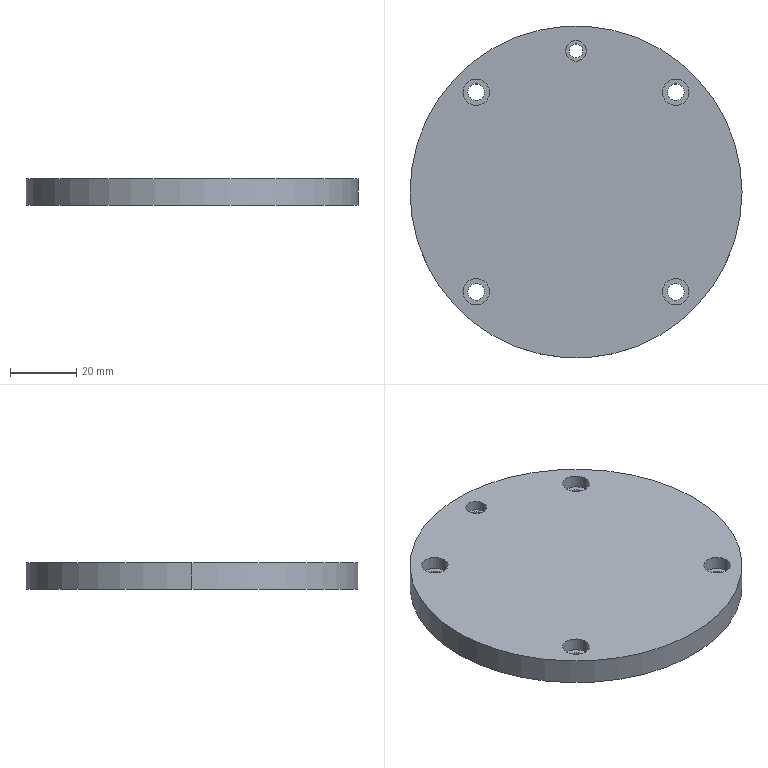Part | SolidWorks | features ICE 4, Extrusion 1 | 1 solid | 29 faces | box 100 x 100 x 8 mm | volume 61554 mm3 | cylinder 22 | plane 7 | commonest cylinder face diameters 5 x8 8 x8 4.2 x2 6.2 x2 100 x2
STEP:
#1=CARTESIAN_POINT('',(-2.1,42.5,0.));
#2=VERTEX_POINT('',#1);
#3=CARTESIAN_POINT('',(2.1,42.5,0.));
#4=VERTEX_POINT('',#3);
#5=CARTESIAN_POINT('',(0.,42.5,0.));
#6=DIRECTION('',(0.,0.,1.));
#7=DIRECTION('',(1.,0.,0.));
#8=AXIS2_PLACEMENT_3D('',#5,#6,#7);
#9=CIRCLE('',#8,2.1);
#10=EDGE_CURVE('',#2,#4,#9,.T.);
#11=ORIENTED_EDGE('',*,*,#10,.F.);
#12=CARTESIAN_POINT('',(-2.1,42.5,5.));
#13=VERTEX_POINT('',#12);
#14=CARTESIAN_POINT('',(-2.1,42.5,0.));
#15=DIRECTION('',(0.,0.,1.));
#16=VECTOR('',#15,1000.);
#17=LINE('',#14,#16);
#18=EDGE_CURVE('',#2,#13,#17,.T.);
#19=ORIENTED_EDGE('',*,*,#18,.T.);
#20=CARTESIAN_POINT('',(2.1,42.5,5.));
#21=VERTEX_POINT('',#20);
#22=CARTESIAN_POINT('',(0.,42.5,5.));
#23=DIRECTION('',(0.,0.,1.));
#24=DIRECTION('',(1.,0.,0.));
#25=AXIS2_PLACEMENT_3D('',#22,#23,#24);
#26=CIRCLE('',#25,2.1);
#27=EDGE_CURVE('',#13,#21,#26,.T.);
#28=ORIENTED_EDGE('',*,*,#27,.T.);
#29=CARTESIAN_POINT('',(2.1,42.5,0.));
#30=DIRECTION('',(0.,0.,1.));
#31=VECTOR('',#30,1000.);
#32=LINE('',#29,#31);
#33=EDGE_CURVE('',#4,#21,#32,.T.);
#34=ORIENTED_EDGE('',*,*,#33,.F.);
#35=EDGE_LOOP('',(#11,#19,#28,#34));
#36=FACE_OUTER_BOUND('',#35,.T.);
#37=CARTESIAN_POINT('',(0.,42.5,0.));
#38=DIRECTION('',(0.,0.,1.));
#39=DIRECTION('',(1.,0.,0.));
#40=AXIS2_PLACEMENT_3D('',#37,#38,#39);
#41=CYLINDRICAL_SURFACE('',#40,2.1);
#42=ADVANCED_FACE('',(#36),#41,.F.);
#43=CARTESIAN_POINT('',(27.554,-30.05,0.));
#44=VERTEX_POINT('',#43);
#45=CARTESIAN_POINT('',(32.554,-30.05,0.));
#46=VERTEX_POINT('',#45);
#47=CARTESIAN_POINT('',(30.054,-30.05,0.));
#48=DIRECTION('',(0.,0.,1.));
#49=DIRECTION('',(1.,0.,0.));
#50=AXIS2_PLACEMENT_3D('',#47,#48,#49);
#51=CIRCLE('',#50,2.5);
#52=EDGE_CURVE('',#44,#46,#51,.T.);
#53=ORIENTED_EDGE('',*,*,#52,.F.);
#54=CARTESIAN_POINT('',(27.554,-30.05,4.));
#55=VERTEX_POINT('',#54);
#56=CARTESIAN_POINT('',(27.554,-30.05,0.));
#57=DIRECTION('',(0.,0.,1.));
#58=VECTOR('',#57,1000.);
#59=LINE('',#56,#58);
#60=EDGE_CURVE('',#44,#55,#59,.T.);
#61=ORIENTED_EDGE('',*,*,#60,.T.);
#62=CARTESIAN_POINT('',(32.554,-30.05,4.));
#63=VERTEX_POINT('',#62);
#64=CARTESIAN_POINT('',(30.054,-30.05,4.));
#65=DIRECTION('',(0.,0.,1.));
#66=DIRECTION('',(1.,0.,0.));
#67=AXIS2_PLACEMENT_3D('',#64,#65,#66);
#68=CIRCLE('',#67,2.5);
#69=EDGE_CURVE('',#55,#63,#68,.T.);
#70=ORIENTED_EDGE('',*,*,#69,.T.);
#71=CARTESIAN_POINT('',(32.554,-30.05,0.));
#72=DIRECTION('',(0.,0.,1.));
#73=VECTOR('',#72,1000.);
#74=LINE('',#71,#73);
#75=EDGE_CURVE('',#46,#63,#74,.T.);
#76=ORIENTED_EDGE('',*,*,#75,.F.);
#77=EDGE_LOOP('',(#53,#61,#70,#76));
#78=FACE_OUTER_BOUND('',#77,.T.);
#79=CARTESIAN_POINT('',(30.054,-30.05,0.));
#80=DIRECTION('',(0.,0.,1.));
#81=DIRECTION('',(1.,0.,0.));
#82=AXIS2_PLACEMENT_3D('',#79,#80,#81);
#83=CYLINDRICAL_SURFACE('',#82,2.5);
#84=ADVANCED_FACE('',(#78),#83,.F.);
#85=CARTESIAN_POINT('',(-32.554,-30.05,0.));
#86=VERTEX_POINT('',#85);
#87=CARTESIAN_POINT('',(-27.554,-30.05,0.));
#88=VERTEX_POINT('',#87);
#89=CARTESIAN_POINT('',(-30.054,-30.05,0.));
#90=DIRECTION('',(0.,0.,1.));
#91=DIRECTION('',(1.,0.,0.));
#92=AXIS2_PLACEMENT_3D('',#89,#90,#91);
#93=CIRCLE('',#92,2.5);
#94=EDGE_CURVE('',#86,#88,#93,.T.);
#95=ORIENTED_EDGE('',*,*,#94,.F.);
#96=CARTESIAN_POINT('',(-32.554,-30.05,4.));
#97=VERTEX_POINT('',#96);
#98=CARTESIAN_POINT('',(-32.554,-30.05,0.));
#99=DIRECTION('',(0.,0.,1.));
#100=VECTOR('',#99,1000.);
#101=LINE('',#98,#100);
#102=EDGE_CURVE('',#86,#97,#101,.T.);
#103=ORIENTED_EDGE('',*,*,#102,.T.);
#104=CARTESIAN_POINT('',(-27.554,-30.05,4.));
#105=VERTEX_POINT('',#104);
#106=CARTESIAN_POINT('',(-30.054,-30.05,4.));
#107=DIRECTION('',(0.,0.,1.));
#108=DIRECTION('',(1.,0.,0.));
#109=AXIS2_PLACEMENT_3D('',#106,#107,#108);
#110=CIRCLE('',#109,2.5);
#111=EDGE_CURVE('',#97,#105,#110,.T.);
#112=ORIENTED_EDGE('',*,*,#111,.T.);
#113=CARTESIAN_POINT('',(-27.554,-30.05,0.));
#114=DIRECTION('',(0.,0.,1.));
#115=VECTOR('',#114,1000.);
#116=LINE('',#113,#115);
#117=EDGE_CURVE('',#88,#105,#116,.T.);
#118=ORIENTED_EDGE('',*,*,#117,.F.);
#119=EDGE_LOOP('',(#95,#103,#112,#118));
#120=FACE_OUTER_BOUND('',#119,.T.);
#121=CARTESIAN_POINT('',(-30.054,-30.05,0.));
#122=DIRECTION('',(0.,0.,1.));
#123=DIRECTION('',(1.,0.,0.));
#124=AXIS2_PLACEMENT_3D('',#121,#122,#123);
#125=CYLINDRICAL_SURFACE('',#124,2.5);
#126=ADVANCED_FACE('',(#120),#125,.F.);
#127=CARTESIAN_POINT('',(27.554,30.05,0.));
#128=VERTEX_POINT('',#127);
#129=CARTESIAN_POINT('',(32.554,30.05,0.));
#130=VERTEX_POINT('',#129);
#131=CARTESIAN_POINT('',(30.054,30.05,0.));
#132=DIRECTION('',(0.,0.,1.));
#133=DIRECTION('',(1.,0.,0.));
#134=AXIS2_PLACEMENT_3D('',#131,#132,#133);
#135=CIRCLE('',#134,2.5);
#136=EDGE_CURVE('',#128,#130,#135,.T.);
#137=ORIENTED_EDGE('',*,*,#136,.F.);
#138=CARTESIAN_POINT('',(27.554,30.05,4.));
#139=VERTEX_POINT('',#138);
#140=CARTESIAN_POINT('',(27.554,30.05,0.));
#141=DIRECTION('',(0.,0.,1.));
#142=VECTOR('',#141,1000.);
#143=LINE('',#140,#142);
#144=EDGE_CURVE('',#128,#139,#143,.T.);
#145=ORIENTED_EDGE('',*,*,#144,.T.);
#146=CARTESIAN_POINT('',(32.554,30.05,4.));
#147=VERTEX_POINT('',#146);
#148=CARTESIAN_POINT('',(30.054,30.05,4.));
#149=DIRECTION('',(0.,0.,1.));
#150=DIRECTION('',(1.,0.,0.));
#151=AXIS2_PLACEMENT_3D('',#148,#149,#150);
#152=CIRCLE('',#151,2.5);
#153=EDGE_CURVE('',#139,#147,#152,.T.);
#154=ORIENTED_EDGE('',*,*,#153,.T.);
#155=CARTESIAN_POINT('',(32.554,30.05,0.));
#156=DIRECTION('',(0.,0.,1.));
#157=VECTOR('',#156,1000.);
#158=LINE('',#155,#157);
#159=EDGE_CURVE('',#130,#147,#158,.T.);
#160=ORIENTED_EDGE('',*,*,#159,.F.);
#161=EDGE_LOOP('',(#137,#145,#154,#160));
#162=FACE_OUTER_BOUND('',#161,.T.);
#163=CARTESIAN_POINT('',(30.054,30.05,0.));
#164=DIRECTION('',(0.,0.,1.));
#165=DIRECTION('',(1.,0.,0.));
#166=AXIS2_PLACEMENT_3D('',#163,#164,#165);
#167=CYLINDRICAL_SURFACE('',#166,2.5);
#168=ADVANCED_FACE('',(#162),#167,.F.);
#169=CARTESIAN_POINT('',(-32.554,30.05,0.));
#170=VERTEX_POINT('',#169);
#171=CARTESIAN_POINT('',(-27.554,30.05,0.));
#172=VERTEX_POINT('',#171);
#173=CARTESIAN_POINT('',(-30.054,30.05,0.));
#174=DIRECTION('',(0.,0.,1.));
#175=DIRECTION('',(1.,0.,0.));
#176=AXIS2_PLACEMENT_3D('',#173,#174,#175);
#177=CIRCLE('',#176,2.5);
#178=EDGE_CURVE('',#170,#172,#177,.T.);
#179=ORIENTED_EDGE('',*,*,#178,.F.);
#180=CARTESIAN_POINT('',(-32.554,30.05,4.));
#181=VERTEX_POINT('',#180);
#182=CARTESIAN_POINT('',(-32.554,30.05,0.));
#183=DIRECTION('',(0.,0.,1.));
#184=VECTOR('',#183,1000.);
#185=LINE('',#182,#184);
#186=EDGE_CURVE('',#170,#181,#185,.T.);
#187=ORIENTED_EDGE('',*,*,#186,.T.);
#188=CARTESIAN_POINT('',(-27.554,30.05,4.));
#189=VERTEX_POINT('',#188);
#190=CARTESIAN_POINT('',(-30.054,30.05,4.));
#191=DIRECTION('',(0.,0.,1.));
#192=DIRECTION('',(1.,0.,0.));
#193=AXIS2_PLACEMENT_3D('',#190,#191,#192);
#194=CIRCLE('',#193,2.5);
#195=EDGE_CURVE('',#181,#189,#194,.T.);
#196=ORIENTED_EDGE('',*,*,#195,.T.);
#197=CARTESIAN_POINT('',(-27.554,30.05,0.));
#198=DIRECTION('',(0.,0.,1.));
#199=VECTOR('',#198,1000.);
#200=LINE('',#197,#199);
#201=EDGE_CURVE('',#172,#189,#200,.T.);
#202=ORIENTED_EDGE('',*,*,#201,.F.);
#203=EDGE_LOOP('',(#179,#187,#196,#202));
#204=FACE_OUTER_BOUND('',#203,.T.);
#205=CARTESIAN_POINT('',(-30.054,30.05,0.));
#206=DIRECTION('',(0.,0.,1.));
#207=DIRECTION('',(1.,0.,0.));
#208=AXIS2_PLACEMENT_3D('',#205,#206,#207);
#209=CYLINDRICAL_SURFACE('',#208,2.5);
#210=ADVANCED_FACE('',(#204),#209,.F.);
#211=CARTESIAN_POINT('',(-3.1,42.5,5.));
#212=VERTEX_POINT('',#211);
#213=CARTESIAN_POINT('',(3.1,42.5,5.));
#214=VERTEX_POINT('',#213);
#215=CARTESIAN_POINT('',(0.,42.5,5.));
#216=DIRECTION('',(0.,0.,1.));
#217=DIRECTION('',(1.,0.,0.));
#218=AXIS2_PLACEMENT_3D('',#215,#216,#217);
#219=CIRCLE('',#218,3.1);
#220=EDGE_CURVE('',#212,#214,#219,.T.);
#221=ORIENTED_EDGE('',*,*,#220,.F.);
#222=CARTESIAN_POINT('',(-3.1,42.5,8.));
#223=VERTEX_POINT('',#222);
#224=CARTESIAN_POINT('',(-3.1,42.5,5.));
#225=DIRECTION('',(0.,0.,1.));
#226=VECTOR('',#225,1000.);
#227=LINE('',#224,#226);
#228=EDGE_CURVE('',#212,#223,#227,.T.);
#229=ORIENTED_EDGE('',*,*,#228,.T.);
#230=CARTESIAN_POINT('',(3.1,42.5,8.));
#231=VERTEX_POINT('',#230);
#232=CARTESIAN_POINT('',(0.,42.5,8.));
#233=DIRECTION('',(0.,0.,1.));
#234=DIRECTION('',(1.,0.,0.));
#235=AXIS2_PLACEMENT_3D('',#232,#233,#234);
#236=CIRCLE('',#235,3.1);
#237=EDGE_CURVE('',#223,#231,#236,.T.);
#238=ORIENTED_EDGE('',*,*,#237,.T.);
#239=CARTESIAN_POINT('',(3.1,42.5,5.));
#240=DIRECTION('',(0.,0.,1.));
#241=VECTOR('',#240,1000.);
#242=LINE('',#239,#241);
#243=EDGE_CURVE('',#214,#231,#242,.T.);
#244=ORIENTED_EDGE('',*,*,#243,.F.);
#245=EDGE_LOOP('',(#221,#229,#238,#244));
#246=FACE_OUTER_BOUND('',#245,.T.);
#247=CARTESIAN_POINT('',(0.,42.5,5.));
#248=DIRECTION('',(0.,0.,1.));
#249=DIRECTION('',(1.,0.,0.));
#250=AXIS2_PLACEMENT_3D('',#247,#248,#249);
#251=CYLINDRICAL_SURFACE('',#250,3.1);
#252=ADVANCED_FACE('',(#246),#251,.F.);
#253=CARTESIAN_POINT('',(26.054,-30.05,4.));
#254=VERTEX_POINT('',#253);
#255=CARTESIAN_POINT('',(34.054,-30.05,4.));
#256=VERTEX_POINT('',#255);
#257=CARTESIAN_POINT('',(30.054,-30.05,4.));
#258=DIRECTION('',(0.,0.,1.));
#259=DIRECTION('',(1.,0.,0.));
#260=AXIS2_PLACEMENT_3D('',#257,#258,#259);
#261=CIRCLE('',#260,4.);
#262=EDGE_CURVE('',#254,#256,#261,.T.);
#263=ORIENTED_EDGE('',*,*,#262,.F.);
#264=CARTESIAN_POINT('',(26.054,-30.05,8.));
#265=VERTEX_POINT('',#264);
#266=CARTESIAN_POINT('',(26.054,-30.05,4.));
#267=DIRECTION('',(0.,0.,1.));
#268=VECTOR('',#267,1000.);
#269=LINE('',#266,#268);
#270=EDGE_CURVE('',#254,#265,#269,.T.);
#271=ORIENTED_EDGE('',*,*,#270,.T.);
#272=CARTESIAN_POINT('',(34.054,-30.05,8.));
#273=VERTEX_POINT('',#272);
#274=CARTESIAN_POINT('',(30.054,-30.05,8.));
#275=DIRECTION('',(0.,0.,1.));
#276=DIRECTION('',(1.,0.,0.));
#277=AXIS2_PLACEMENT_3D('',#274,#275,#276);
#278=CIRCLE('',#277,4.);
#279=EDGE_CURVE('',#265,#273,#278,.T.);
#280=ORIENTED_EDGE('',*,*,#279,.T.);
#281=CARTESIAN_POINT('',(34.054,-30.05,4.));
#282=DIRECTION('',(0.,0.,1.));
#283=VECTOR('',#282,1000.);
#284=LINE('',#281,#283);
#285=EDGE_CURVE('',#256,#273,#284,.T.);
#286=ORIENTED_EDGE('',*,*,#285,.F.);
#287=EDGE_LOOP('',(#263,#271,#280,#286));
#288=FACE_OUTER_BOUND('',#287,.T.);
#289=CARTESIAN_POINT('',(30.054,-30.05,4.));
#290=DIRECTION('',(0.,0.,1.));
#291=DIRECTION('',(1.,0.,0.));
#292=AXIS2_PLACEMENT_3D('',#289,#290,#291);
#293=CYLINDRICAL_SURFACE('',#292,4.);
#294=ADVANCED_FACE('',(#288),#293,.F.);
#295=CARTESIAN_POINT('',(-34.054,-30.05,4.));
#296=VERTEX_POINT('',#295);
#297=CARTESIAN_POINT('',(-26.054,-30.05,4.));
#298=VERTEX_POINT('',#297);
#299=CARTESIAN_POINT('',(-30.054,-30.05,4.));
#300=DIRECTION('',(0.,0.,1.));
#301=DIRECTION('',(1.,0.,0.));
#302=AXIS2_PLACEMENT_3D('',#299,#300,#301);
#303=CIRCLE('',#302,4.);
#304=EDGE_CURVE('',#296,#298,#303,.T.);
#305=ORIENTED_EDGE('',*,*,#304,.F.);
#306=CARTESIAN_POINT('',(-34.054,-30.05,8.));
#307=VERTEX_POINT('',#306);
#308=CARTESIAN_POINT('',(-34.054,-30.05,4.));
#309=DIRECTION('',(0.,0.,1.));
#310=VECTOR('',#309,1000.);
#311=LINE('',#308,#310);
#312=EDGE_CURVE('',#296,#307,#311,.T.);
#313=ORIENTED_EDGE('',*,*,#312,.T.);
#314=CARTESIAN_POINT('',(-26.054,-30.05,8.));
#315=VERTEX_POINT('',#314);
#316=CARTESIAN_POINT('',(-30.054,-30.05,8.));
#317=DIRECTION('',(0.,0.,1.));
#318=DIRECTION('',(1.,0.,0.));
#319=AXIS2_PLACEMENT_3D('',#316,#317,#318);
#320=CIRCLE('',#319,4.);
#321=EDGE_CURVE('',#307,#315,#320,.T.);
#322=ORIENTED_EDGE('',*,*,#321,.T.);
#323=CARTESIAN_POINT('',(-26.054,-30.05,4.));
#324=DIRECTION('',(0.,0.,1.));
#325=VECTOR('',#324,1000.);
#326=LINE('',#323,#325);
#327=EDGE_CURVE('',#298,#315,#326,.T.);
#328=ORIENTED_EDGE('',*,*,#327,.F.);
#329=EDGE_LOOP('',(#305,#313,#322,#328));
#330=FACE_OUTER_BOUND('',#329,.T.);
#331=CARTESIAN_POINT('',(-30.054,-30.05,4.));
#332=DIRECTION('',(0.,0.,1.));
#333=DIRECTION('',(1.,0.,0.));
#334=AXIS2_PLACEMENT_3D('',#331,#332,#333);
#335=CYLINDRICAL_SURFACE('',#334,4.);
#336=ADVANCED_FACE('',(#330),#335,.F.);
#337=CARTESIAN_POINT('',(26.054,30.05,4.));
#338=VERTEX_POINT('',#337);
#339=CARTESIAN_POINT('',(34.054,30.05,4.));
#340=VERTEX_POINT('',#339);
#341=CARTESIAN_POINT('',(30.054,30.05,4.));
#342=DIRECTION('',(0.,0.,1.));
#343=DIRECTION('',(1.,0.,0.));
#344=AXIS2_PLACEMENT_3D('',#341,#342,#343);
#345=CIRCLE('',#344,4.);
#346=EDGE_CURVE('',#338,#340,#345,.T.);
#347=ORIENTED_EDGE('',*,*,#346,.F.);
#348=CARTESIAN_POINT('',(26.054,30.05,8.));
#349=VERTEX_POINT('',#348);
#350=CARTESIAN_POINT('',(26.054,30.05,4.));
#351=DIRECTION('',(0.,0.,1.));
#352=VECTOR('',#351,1000.);
#353=LINE('',#350,#352);
#354=EDGE_CURVE('',#338,#349,#353,.T.);
#355=ORIENTED_EDGE('',*,*,#354,.T.);
#356=CARTESIAN_POINT('',(34.054,30.05,8.));
#357=VERTEX_POINT('',#356);
#358=CARTESIAN_POINT('',(30.054,30.05,8.));
#359=DIRECTION('',(0.,0.,1.));
#360=DIRECTION('',(1.,0.,0.));
#361=AXIS2_PLACEMENT_3D('',#358,#359,#360);
#362=CIRCLE('',#361,4.);
#363=EDGE_CURVE('',#349,#357,#362,.T.);
#364=ORIENTED_EDGE('',*,*,#363,.T.);
#365=CARTESIAN_POINT('',(34.054,30.05,4.));
#366=DIRECTION('',(0.,0.,1.));
#367=VECTOR('',#366,1000.);
#368=LINE('',#365,#367);
#369=EDGE_CURVE('',#340,#357,#368,.T.);
#370=ORIENTED_EDGE('',*,*,#369,.F.);
#371=EDGE_LOOP('',(#347,#355,#364,#370));
#372=FACE_OUTER_BOUND('',#371,.T.);
#373=CARTESIAN_POINT('',(30.054,30.05,4.));
#374=DIRECTION('',(0.,0.,1.));
#375=DIRECTION('',(1.,0.,0.));
#376=AXIS2_PLACEMENT_3D('',#373,#374,#375);
#377=CYLINDRICAL_SURFACE('',#376,4.);
#378=ADVANCED_FACE('',(#372),#377,.F.);
#379=CARTESIAN_POINT('',(-34.054,30.05,4.));
#380=VERTEX_POINT('',#379);
#381=CARTESIAN_POINT('',(-26.054,30.05,4.));
#382=VERTEX_POINT('',#381);
#383=CARTESIAN_POINT('',(-30.054,30.05,4.));
#384=DIRECTION('',(0.,0.,1.));
#385=DIRECTION('',(1.,0.,0.));
#386=AXIS2_PLACEMENT_3D('',#383,#384,#385);
#387=CIRCLE('',#386,4.);
#388=EDGE_CURVE('',#380,#382,#387,.T.);
#389=ORIENTED_EDGE('',*,*,#388,.F.);
#390=CARTESIAN_POINT('',(-34.054,30.05,8.));
#391=VERTEX_POINT('',#390);
#392=CARTESIAN_POINT('',(-34.054,30.05,4.));
#393=DIRECTION('',(0.,0.,1.));
#394=VECTOR('',#393,1000.);
#395=LINE('',#392,#394);
#396=EDGE_CURVE('',#380,#391,#395,.T.);
#397=ORIENTED_EDGE('',*,*,#396,.T.);
#398=CARTESIAN_POINT('',(-26.054,30.05,8.));
#399=VERTEX_POINT('',#398);
#400=CARTESIAN_POINT('',(-30.054,30.05,8.));
#401=DIRECTION('',(0.,0.,1.));
#402=DIRECTION('',(1.,0.,0.));
#403=AXIS2_PLACEMENT_3D('',#400,#401,#402);
#404=CIRCLE('',#403,4.);
#405=EDGE_CURVE('',#391,#399,#404,.T.);
#406=ORIENTED_EDGE('',*,*,#405,.T.);
#407=CARTESIAN_POINT('',(-26.054,30.05,4.));
#408=DIRECTION('',(0.,0.,1.));
#409=VECTOR('',#408,1000.);
#410=LINE('',#407,#409);
#411=EDGE_CURVE('',#382,#399,#410,.T.);
#412=ORIENTED_EDGE('',*,*,#411,.F.);
#413=EDGE_LOOP('',(#389,#397,#406,#412));
#414=FACE_OUTER_BOUND('',#413,.T.);
#415=CARTESIAN_POINT('',(-30.054,30.05,4.));
#416=DIRECTION('',(0.,0.,1.));
#417=DIRECTION('',(1.,0.,0.));
#418=AXIS2_PLACEMENT_3D('',#415,#416,#417);
#419=CYLINDRICAL_SURFACE('',#418,4.);
#420=ADVANCED_FACE('',(#414),#419,.F.);
#421=CARTESIAN_POINT('',(50.,0.,8.));
#422=VERTEX_POINT('',#421);
#423=CARTESIAN_POINT('',(-50.,0.,8.));
#424=VERTEX_POINT('',#423);
#425=CARTESIAN_POINT('',(0.,0.,8.));
#426=DIRECTION('',(0.,0.,1.));
#427=DIRECTION('',(1.,0.,0.));
#428=AXIS2_PLACEMENT_3D('',#425,#426,#427);
#429=CIRCLE('',#428,50.);
#430=EDGE_CURVE('',#422,#424,#429,.T.);
#431=ORIENTED_EDGE('',*,*,#430,.F.);
#432=CARTESIAN_POINT('',(50.,0.,0.));
#433=VERTEX_POINT('',#432);
#434=CARTESIAN_POINT('',(50.,0.,8.));
#435=DIRECTION('',(0.,0.,-1.));
#436=VECTOR('',#435,1000.);
#437=LINE('',#434,#436);
#438=EDGE_CURVE('',#422,#433,#437,.T.);
#439=ORIENTED_EDGE('',*,*,#438,.T.);
#440=CARTESIAN_POINT('',(-50.,0.,0.));
#441=VERTEX_POINT('',#440);
#442=CARTESIAN_POINT('',(0.,0.,0.));
#443=DIRECTION('',(0.,0.,1.));
#444=DIRECTION('',(1.,0.,0.));
#445=AXIS2_PLACEMENT_3D('',#442,#443,#444);
#446=CIRCLE('',#445,50.);
#447=EDGE_CURVE('',#433,#441,#446,.T.);
#448=ORIENTED_EDGE('',*,*,#447,.T.);
#449=CARTESIAN_POINT('',(-50.,0.,8.));
#450=DIRECTION('',(0.,0.,-1.));
#451=VECTOR('',#450,1000.);
#452=LINE('',#449,#451);
#453=EDGE_CURVE('',#424,#441,#452,.T.);
#454=ORIENTED_EDGE('',*,*,#453,.F.);
#455=EDGE_LOOP('',(#431,#439,#448,#454));
#456=FACE_OUTER_BOUND('',#455,.T.);
#457=CARTESIAN_POINT('',(0.,0.,8.));
#458=DIRECTION('',(0.,0.,-1.));
#459=DIRECTION('',(-1.,0.,0.));
#460=AXIS2_PLACEMENT_3D('',#457,#458,#459);
#461=CYLINDRICAL_SURFACE('',#460,50.);
#462=ADVANCED_FACE('',(#456),#461,.T.);
#463=ORIENTED_EDGE('',*,*,#438,.F.);
#464=CARTESIAN_POINT('',(0.,0.,8.));
#465=DIRECTION('',(0.,0.,1.));
#466=DIRECTION('',(1.,0.,0.));
#467=AXIS2_PLACEMENT_3D('',#464,#465,#466);
#468=CIRCLE('',#467,50.);
#469=EDGE_CURVE('',#424,#422,#468,.T.);
#470=ORIENTED_EDGE('',*,*,#469,.F.);
#471=ORIENTED_EDGE('',*,*,#453,.T.);
#472=CARTESIAN_POINT('',(0.,0.,0.));
#473=DIRECTION('',(0.,0.,1.));
#474=DIRECTION('',(1.,0.,0.));
#475=AXIS2_PLACEMENT_3D('',#472,#473,#474);
#476=CIRCLE('',#475,50.);
#477=EDGE_CURVE('',#441,#433,#476,.T.);
#478=ORIENTED_EDGE('',*,*,#477,.T.);
#479=EDGE_LOOP('',(#463,#470,#471,#478));
#480=FACE_OUTER_BOUND('',#479,.T.);
#481=CARTESIAN_POINT('',(0.,0.,8.));
#482=DIRECTION('',(0.,0.,-1.));
#483=DIRECTION('',(-1.,0.,0.));
#484=AXIS2_PLACEMENT_3D('',#481,#482,#483);
#485=CYLINDRICAL_SURFACE('',#484,50.);
#486=ADVANCED_FACE('',(#480),#485,.T.);
#487=CARTESIAN_POINT('',(0.,42.5,8.));
#488=DIRECTION('',(0.,0.,1.));
#489=DIRECTION('',(1.,0.,0.));
#490=AXIS2_PLACEMENT_3D('',#487,#488,#489);
#491=CIRCLE('',#490,3.1);
#492=EDGE_CURVE('',#231,#223,#491,.T.);
#493=ORIENTED_EDGE('',*,*,#492,.F.);
#494=ORIENTED_EDGE('',*,*,#237,.F.);
#495=EDGE_LOOP('',(#493,#494));
#496=FACE_BOUND('',#495,.T.);
#497=CARTESIAN_POINT('',(30.054,-30.05,8.));
#498=DIRECTION('',(0.,0.,1.));
#499=DIRECTION('',(1.,0.,0.));
#500=AXIS2_PLACEMENT_3D('',#497,#498,#499);
#501=CIRCLE('',#500,4.);
#502=EDGE_CURVE('',#273,#265,#501,.T.);
#503=ORIENTED_EDGE('',*,*,#502,.F.);
#504=ORIENTED_EDGE('',*,*,#279,.F.);
#505=EDGE_LOOP('',(#503,#504));
#506=FACE_BOUND('',#505,.T.);
#507=CARTESIAN_POINT('',(-30.054,-30.05,8.));
#508=DIRECTION('',(0.,0.,1.));
#509=DIRECTION('',(1.,0.,0.));
#510=AXIS2_PLACEMENT_3D('',#507,#508,#509);
#511=CIRCLE('',#510,4.);
#512=EDGE_CURVE('',#315,#307,#511,.T.);
#513=ORIENTED_EDGE('',*,*,#512,.F.);
#514=ORIENTED_EDGE('',*,*,#321,.F.);
#515=EDGE_LOOP('',(#513,#514));
#516=FACE_BOUND('',#515,.T.);
#517=CARTESIAN_POINT('',(30.054,30.05,8.));
#518=DIRECTION('',(0.,0.,1.));
#519=DIRECTION('',(1.,0.,0.));
#520=AXIS2_PLACEMENT_3D('',#517,#518,#519);
#521=CIRCLE('',#520,4.);
#522=EDGE_CURVE('',#357,#349,#521,.T.);
#523=ORIENTED_EDGE('',*,*,#522,.F.);
#524=ORIENTED_EDGE('',*,*,#363,.F.);
#525=EDGE_LOOP('',(#523,#524));
#526=FACE_BOUND('',#525,.T.);
#527=CARTESIAN_POINT('',(-30.054,30.05,8.));
#528=DIRECTION('',(0.,0.,1.));
#529=DIRECTION('',(1.,0.,0.));
#530=AXIS2_PLACEMENT_3D('',#527,#528,#529);
#531=CIRCLE('',#530,4.);
#532=EDGE_CURVE('',#399,#391,#531,.T.);
#533=ORIENTED_EDGE('',*,*,#532,.F.);
#534=ORIENTED_EDGE('',*,*,#405,.F.);
#535=EDGE_LOOP('',(#533,#534));
#536=FACE_BOUND('',#535,.T.);
#537=ORIENTED_EDGE('',*,*,#469,.T.);
#538=ORIENTED_EDGE('',*,*,#430,.T.);
#539=EDGE_LOOP('',(#537,#538));
#540=FACE_OUTER_BOUND('',#539,.T.);
#541=CARTESIAN_POINT('',(0.,0.,8.));
#542=DIRECTION('',(0.,0.,1.));
#543=DIRECTION('',(1.,0.,0.));
#544=AXIS2_PLACEMENT_3D('',#541,#542,#543);
#545=PLANE('',#544);
#546=ADVANCED_FACE('',(#496,#506,#516,#526,#536,#540),#545,.T.);
#547=CARTESIAN_POINT('',(0.,42.5,0.));
#548=DIRECTION('',(0.,0.,1.));
#549=DIRECTION('',(1.,0.,0.));
#550=AXIS2_PLACEMENT_3D('',#547,#548,#549);
#551=CIRCLE('',#550,2.1);
#552=EDGE_CURVE('',#4,#2,#551,.T.);
#553=ORIENTED_EDGE('',*,*,#552,.T.);
#554=ORIENTED_EDGE('',*,*,#10,.T.);
#555=EDGE_LOOP('',(#553,#554));
#556=FACE_BOUND('',#555,.T.);
#557=CARTESIAN_POINT('',(30.054,-30.05,0.));
#558=DIRECTION('',(0.,0.,1.));
#559=DIRECTION('',(1.,0.,0.));
#560=AXIS2_PLACEMENT_3D('',#557,#558,#559);
#561=CIRCLE('',#560,2.5);
#562=EDGE_CURVE('',#46,#44,#561,.T.);
#563=ORIENTED_EDGE('',*,*,#562,.T.);
#564=ORIENTED_EDGE('',*,*,#52,.T.);
#565=EDGE_LOOP('',(#563,#564));
#566=FACE_BOUND('',#565,.T.);
#567=CARTESIAN_POINT('',(-30.054,-30.05,0.));
#568=DIRECTION('',(0.,0.,1.));
#569=DIRECTION('',(1.,0.,0.));
#570=AXIS2_PLACEMENT_3D('',#567,#568,#569);
#571=CIRCLE('',#570,2.5);
#572=EDGE_CURVE('',#88,#86,#571,.T.);
#573=ORIENTED_EDGE('',*,*,#572,.T.);
#574=ORIENTED_EDGE('',*,*,#94,.T.);
#575=EDGE_LOOP('',(#573,#574));
#576=FACE_BOUND('',#575,.T.);
#577=CARTESIAN_POINT('',(30.054,30.05,0.));
#578=DIRECTION('',(0.,0.,1.));
#579=DIRECTION('',(1.,0.,0.));
#580=AXIS2_PLACEMENT_3D('',#577,#578,#579);
#581=CIRCLE('',#580,2.5);
#582=EDGE_CURVE('',#130,#128,#581,.T.);
#583=ORIENTED_EDGE('',*,*,#582,.T.);
#584=ORIENTED_EDGE('',*,*,#136,.T.);
#585=EDGE_LOOP('',(#583,#584));
#586=FACE_BOUND('',#585,.T.);
#587=CARTESIAN_POINT('',(-30.054,30.05,0.));
#588=DIRECTION('',(0.,0.,1.));
#589=DIRECTION('',(1.,0.,0.));
#590=AXIS2_PLACEMENT_3D('',#587,#588,#589);
#591=CIRCLE('',#590,2.5);
#592=EDGE_CURVE('',#172,#170,#591,.T.);
#593=ORIENTED_EDGE('',*,*,#592,.T.);
#594=ORIENTED_EDGE('',*,*,#178,.T.);
#595=EDGE_LOOP('',(#593,#594));
#596=FACE_BOUND('',#595,.T.);
#597=ORIENTED_EDGE('',*,*,#477,.F.);
#598=ORIENTED_EDGE('',*,*,#447,.F.);
#599=EDGE_LOOP('',(#597,#598));
#600=FACE_OUTER_BOUND('',#599,.T.);
#601=CARTESIAN_POINT('',(0.,0.,0.));
#602=DIRECTION('',(0.,0.,1.));
#603=DIRECTION('',(1.,0.,0.));
#604=AXIS2_PLACEMENT_3D('',#601,#602,#603);
#605=PLANE('',#604);
#606=ADVANCED_FACE('',(#556,#566,#576,#586,#596,#600),#605,.F.);
#607=ORIENTED_EDGE('',*,*,#396,.F.);
#608=CARTESIAN_POINT('',(-30.054,30.05,4.));
#609=DIRECTION('',(0.,0.,1.));
#610=DIRECTION('',(1.,0.,0.));
#611=AXIS2_PLACEMENT_3D('',#608,#609,#610);
#612=CIRCLE('',#611,4.);
#613=EDGE_CURVE('',#382,#380,#612,.T.);
#614=ORIENTED_EDGE('',*,*,#613,.F.);
#615=ORIENTED_EDGE('',*,*,#411,.T.);
#616=ORIENTED_EDGE('',*,*,#532,.T.);
#617=EDGE_LOOP('',(#607,#614,#615,#616));
#618=FACE_OUTER_BOUND('',#617,.T.);
#619=CARTESIAN_POINT('',(-30.054,30.05,4.));
#620=DIRECTION('',(0.,0.,1.));
#621=DIRECTION('',(1.,0.,0.));
#622=AXIS2_PLACEMENT_3D('',#619,#620,#621);
#623=CYLINDRICAL_SURFACE('',#622,4.);
#624=ADVANCED_FACE('',(#618),#623,.F.);
#625=CARTESIAN_POINT('',(-30.054,30.05,4.));
#626=DIRECTION('',(0.,0.,1.));
#627=DIRECTION('',(1.,0.,0.));
#628=AXIS2_PLACEMENT_3D('',#625,#626,#627);
#629=CIRCLE('',#628,2.5);
#630=EDGE_CURVE('',#189,#181,#629,.T.);
#631=ORIENTED_EDGE('',*,*,#630,.F.);
#632=ORIENTED_EDGE('',*,*,#195,.F.);
#633=EDGE_LOOP('',(#631,#632));
#634=FACE_BOUND('',#633,.T.);
#635=ORIENTED_EDGE('',*,*,#613,.T.);
#636=ORIENTED_EDGE('',*,*,#388,.T.);
#637=EDGE_LOOP('',(#635,#636));
#638=FACE_OUTER_BOUND('',#637,.T.);
#639=CARTESIAN_POINT('',(-30.054,30.05,4.));
#640=DIRECTION('',(0.,0.,1.));
#641=DIRECTION('',(1.,0.,0.));
#642=AXIS2_PLACEMENT_3D('',#639,#640,#641);
#643=PLANE('',#642);
#644=ADVANCED_FACE('',(#634,#638),#643,.T.);
#645=ORIENTED_EDGE('',*,*,#354,.F.);
#646=CARTESIAN_POINT('',(30.054,30.05,4.));
#647=DIRECTION('',(0.,0.,1.));
#648=DIRECTION('',(1.,0.,0.));
#649=AXIS2_PLACEMENT_3D('',#646,#647,#648);
#650=CIRCLE('',#649,4.);
#651=EDGE_CURVE('',#340,#338,#650,.T.);
#652=ORIENTED_EDGE('',*,*,#651,.F.);
#653=ORIENTED_EDGE('',*,*,#369,.T.);
#654=ORIENTED_EDGE('',*,*,#522,.T.);
#655=EDGE_LOOP('',(#645,#652,#653,#654));
#656=FACE_OUTER_BOUND('',#655,.T.);
#657=CARTESIAN_POINT('',(30.054,30.05,4.));
#658=DIRECTION('',(0.,0.,1.));
#659=DIRECTION('',(1.,0.,0.));
#660=AXIS2_PLACEMENT_3D('',#657,#658,#659);
#661=CYLINDRICAL_SURFACE('',#660,4.);
#662=ADVANCED_FACE('',(#656),#661,.F.);
#663=CARTESIAN_POINT('',(30.054,30.05,4.));
#664=DIRECTION('',(0.,0.,1.));
#665=DIRECTION('',(1.,0.,0.));
#666=AXIS2_PLACEMENT_3D('',#663,#664,#665);
#667=CIRCLE('',#666,2.5);
#668=EDGE_CURVE('',#147,#139,#667,.T.);
#669=ORIENTED_EDGE('',*,*,#668,.F.);
#670=ORIENTED_EDGE('',*,*,#153,.F.);
#671=EDGE_LOOP('',(#669,#670));
#672=FACE_BOUND('',#671,.T.);
#673=ORIENTED_EDGE('',*,*,#651,.T.);
#674=ORIENTED_EDGE('',*,*,#346,.T.);
#675=EDGE_LOOP('',(#673,#674));
#676=FACE_OUTER_BOUND('',#675,.T.);
#677=CARTESIAN_POINT('',(30.054,30.05,4.));
#678=DIRECTION('',(0.,0.,1.));
#679=DIRECTION('',(1.,0.,0.));
#680=AXIS2_PLACEMENT_3D('',#677,#678,#679);
#681=PLANE('',#680);
#682=ADVANCED_FACE('',(#672,#676),#681,.T.);
#683=ORIENTED_EDGE('',*,*,#312,.F.);
#684=CARTESIAN_POINT('',(-30.054,-30.05,4.));
#685=DIRECTION('',(0.,0.,1.));
#686=DIRECTION('',(1.,0.,0.));
#687=AXIS2_PLACEMENT_3D('',#684,#685,#686);
#688=CIRCLE('',#687,4.);
#689=EDGE_CURVE('',#298,#296,#688,.T.);
#690=ORIENTED_EDGE('',*,*,#689,.F.);
#691=ORIENTED_EDGE('',*,*,#327,.T.);
#692=ORIENTED_EDGE('',*,*,#512,.T.);
#693=EDGE_LOOP('',(#683,#690,#691,#692));
#694=FACE_OUTER_BOUND('',#693,.T.);
#695=CARTESIAN_POINT('',(-30.054,-30.05,4.));
#696=DIRECTION('',(0.,0.,1.));
#697=DIRECTION('',(1.,0.,0.));
#698=AXIS2_PLACEMENT_3D('',#695,#696,#697);
#699=CYLINDRICAL_SURFACE('',#698,4.);
#700=ADVANCED_FACE('',(#694),#699,.F.);
#701=CARTESIAN_POINT('',(-30.054,-30.05,4.));
#702=DIRECTION('',(0.,0.,1.));
#703=DIRECTION('',(1.,0.,0.));
#704=AXIS2_PLACEMENT_3D('',#701,#702,#703);
#705=CIRCLE('',#704,2.5);
#706=EDGE_CURVE('',#105,#97,#705,.T.);
#707=ORIENTED_EDGE('',*,*,#706,.F.);
#708=ORIENTED_EDGE('',*,*,#111,.F.);
#709=EDGE_LOOP('',(#707,#708));
#710=FACE_BOUND('',#709,.T.);
#711=ORIENTED_EDGE('',*,*,#689,.T.);
#712=ORIENTED_EDGE('',*,*,#304,.T.);
#713=EDGE_LOOP('',(#711,#712));
#714=FACE_OUTER_BOUND('',#713,.T.);
#715=CARTESIAN_POINT('',(-30.054,-30.05,4.));
#716=DIRECTION('',(0.,0.,1.));
#717=DIRECTION('',(1.,0.,0.));
#718=AXIS2_PLACEMENT_3D('',#715,#716,#717);
#719=PLANE('',#718);
#720=ADVANCED_FACE('',(#710,#714),#719,.T.);
#721=ORIENTED_EDGE('',*,*,#270,.F.);
#722=CARTESIAN_POINT('',(30.054,-30.05,4.));
#723=DIRECTION('',(0.,0.,1.));
#724=DIRECTION('',(1.,0.,0.));
#725=AXIS2_PLACEMENT_3D('',#722,#723,#724);
#726=CIRCLE('',#725,4.);
#727=EDGE_CURVE('',#256,#254,#726,.T.);
#728=ORIENTED_EDGE('',*,*,#727,.F.);
#729=ORIENTED_EDGE('',*,*,#285,.T.);
#730=ORIENTED_EDGE('',*,*,#502,.T.);
#731=EDGE_LOOP('',(#721,#728,#729,#730));
#732=FACE_OUTER_BOUND('',#731,.T.);
#733=CARTESIAN_POINT('',(30.054,-30.05,4.));
#734=DIRECTION('',(0.,0.,1.));
#735=DIRECTION('',(1.,0.,0.));
#736=AXIS2_PLACEMENT_3D('',#733,#734,#735);
#737=CYLINDRICAL_SURFACE('',#736,4.);
#738=ADVANCED_FACE('',(#732),#737,.F.);
#739=CARTESIAN_POINT('',(30.054,-30.05,4.));
#740=DIRECTION('',(0.,0.,1.));
#741=DIRECTION('',(1.,0.,0.));
#742=AXIS2_PLACEMENT_3D('',#739,#740,#741);
#743=CIRCLE('',#742,2.5);
#744=EDGE_CURVE('',#63,#55,#743,.T.);
#745=ORIENTED_EDGE('',*,*,#744,.F.);
#746=ORIENTED_EDGE('',*,*,#69,.F.);
#747=EDGE_LOOP('',(#745,#746));
#748=FACE_BOUND('',#747,.T.);
#749=ORIENTED_EDGE('',*,*,#727,.T.);
#750=ORIENTED_EDGE('',*,*,#262,.T.);
#751=EDGE_LOOP('',(#749,#750));
#752=FACE_OUTER_BOUND('',#751,.T.);
#753=CARTESIAN_POINT('',(30.054,-30.05,4.));
#754=DIRECTION('',(0.,0.,1.));
#755=DIRECTION('',(1.,0.,0.));
#756=AXIS2_PLACEMENT_3D('',#753,#754,#755);
#757=PLANE('',#756);
#758=ADVANCED_FACE('',(#748,#752),#757,.T.);
#759=ORIENTED_EDGE('',*,*,#228,.F.);
#760=CARTESIAN_POINT('',(0.,42.5,5.));
#761=DIRECTION('',(0.,0.,1.));
#762=DIRECTION('',(1.,0.,0.));
#763=AXIS2_PLACEMENT_3D('',#760,#761,#762);
#764=CIRCLE('',#763,3.1);
#765=EDGE_CURVE('',#214,#212,#764,.T.);
#766=ORIENTED_EDGE('',*,*,#765,.F.);
#767=ORIENTED_EDGE('',*,*,#243,.T.);
#768=ORIENTED_EDGE('',*,*,#492,.T.);
#769=EDGE_LOOP('',(#759,#766,#767,#768));
#770=FACE_OUTER_BOUND('',#769,.T.);
#771=CARTESIAN_POINT('',(0.,42.5,5.));
#772=DIRECTION('',(0.,0.,1.));
#773=DIRECTION('',(1.,0.,0.));
#774=AXIS2_PLACEMENT_3D('',#771,#772,#773);
#775=CYLINDRICAL_SURFACE('',#774,3.1);
#776=ADVANCED_FACE('',(#770),#775,.F.);
#777=CARTESIAN_POINT('',(0.,42.5,5.));
#778=DIRECTION('',(0.,0.,1.));
#779=DIRECTION('',(1.,0.,0.));
#780=AXIS2_PLACEMENT_3D('',#777,#778,#779);
#781=CIRCLE('',#780,2.1);
#782=EDGE_CURVE('',#21,#13,#781,.T.);
#783=ORIENTED_EDGE('',*,*,#782,.F.);
#784=ORIENTED_EDGE('',*,*,#27,.F.);
#785=EDGE_LOOP('',(#783,#784));
#786=FACE_BOUND('',#785,.T.);
#787=ORIENTED_EDGE('',*,*,#765,.T.);
#788=ORIENTED_EDGE('',*,*,#220,.T.);
#789=EDGE_LOOP('',(#787,#788));
#790=FACE_OUTER_BOUND('',#789,.T.);
#791=CARTESIAN_POINT('',(0.,42.5,5.));
#792=DIRECTION('',(0.,0.,1.));
#793=DIRECTION('',(1.,0.,0.));
#794=AXIS2_PLACEMENT_3D('',#791,#792,#793);
#795=PLANE('',#794);
#796=ADVANCED_FACE('',(#786,#790),#795,.T.);
#797=ORIENTED_EDGE('',*,*,#186,.F.);
#798=ORIENTED_EDGE('',*,*,#592,.F.);
#799=ORIENTED_EDGE('',*,*,#201,.T.);
#800=ORIENTED_EDGE('',*,*,#630,.T.);
#801=EDGE_LOOP('',(#797,#798,#799,#800));
#802=FACE_OUTER_BOUND('',#801,.T.);
#803=CARTESIAN_POINT('',(-30.054,30.05,0.));
#804=DIRECTION('',(0.,0.,1.));
#805=DIRECTION('',(1.,0.,0.));
#806=AXIS2_PLACEMENT_3D('',#803,#804,#805);
#807=CYLINDRICAL_SURFACE('',#806,2.5);
#808=ADVANCED_FACE('',(#802),#807,.F.);
#809=ORIENTED_EDGE('',*,*,#144,.F.);
#810=ORIENTED_EDGE('',*,*,#582,.F.);
#811=ORIENTED_EDGE('',*,*,#159,.T.);
#812=ORIENTED_EDGE('',*,*,#668,.T.);
#813=EDGE_LOOP('',(#809,#810,#811,#812));
#814=FACE_OUTER_BOUND('',#813,.T.);
#815=CARTESIAN_POINT('',(30.054,30.05,0.));
#816=DIRECTION('',(0.,0.,1.));
#817=DIRECTION('',(1.,0.,0.));
#818=AXIS2_PLACEMENT_3D('',#815,#816,#817);
#819=CYLINDRICAL_SURFACE('',#818,2.5);
#820=ADVANCED_FACE('',(#814),#819,.F.);
#821=ORIENTED_EDGE('',*,*,#102,.F.);
#822=ORIENTED_EDGE('',*,*,#572,.F.);
#823=ORIENTED_EDGE('',*,*,#117,.T.);
#824=ORIENTED_EDGE('',*,*,#706,.T.);
#825=EDGE_LOOP('',(#821,#822,#823,#824));
#826=FACE_OUTER_BOUND('',#825,.T.);
#827=CARTESIAN_POINT('',(-30.054,-30.05,0.));
#828=DIRECTION('',(0.,0.,1.));
#829=DIRECTION('',(1.,0.,0.));
#830=AXIS2_PLACEMENT_3D('',#827,#828,#829);
#831=CYLINDRICAL_SURFACE('',#830,2.5);
#832=ADVANCED_FACE('',(#826),#831,.F.);
#833=ORIENTED_EDGE('',*,*,#60,.F.);
#834=ORIENTED_EDGE('',*,*,#562,.F.);
#835=ORIENTED_EDGE('',*,*,#75,.T.);
#836=ORIENTED_EDGE('',*,*,#744,.T.);
#837=EDGE_LOOP('',(#833,#834,#835,#836));
#838=FACE_OUTER_BOUND('',#837,.T.);
#839=CARTESIAN_POINT('',(30.054,-30.05,0.));
#840=DIRECTION('',(0.,0.,1.));
#841=DIRECTION('',(1.,0.,0.));
#842=AXIS2_PLACEMENT_3D('',#839,#840,#841);
#843=CYLINDRICAL_SURFACE('',#842,2.5);
#844=ADVANCED_FACE('',(#838),#843,.F.);
#845=ORIENTED_EDGE('',*,*,#18,.F.);
#846=ORIENTED_EDGE('',*,*,#552,.F.);
#847=ORIENTED_EDGE('',*,*,#33,.T.);
#848=ORIENTED_EDGE('',*,*,#782,.T.);
#849=EDGE_LOOP('',(#845,#846,#847,#848));
#850=FACE_OUTER_BOUND('',#849,.T.);
#851=CARTESIAN_POINT('',(0.,42.5,0.));
#852=DIRECTION('',(0.,0.,1.));
#853=DIRECTION('',(1.,0.,0.));
#854=AXIS2_PLACEMENT_3D('',#851,#852,#853);
#855=CYLINDRICAL_SURFACE('',#854,2.1);
#856=ADVANCED_FACE('',(#850),#855,.F.);
#857=CLOSED_SHELL('',(#42,#84,#126,#168,#210,#252,#294,#336,#378,#420,#462,#486,#546,#606,#624,#644,#662,#682,#700,#720,#738,#758,#776,#796,#808,#820,#832,#844,#856));
#858=MANIFOLD_SOLID_BREP('',#857);
#859=CARTESIAN_POINT('',(0.,0.,0.));
#860=DIRECTION('',(0.,0.,1.));
#861=DIRECTION('',(1.,0.,0.));
#862=AXIS2_PLACEMENT_3D('',#859,#860,#861);
#863=(LENGTH_UNIT()NAMED_UNIT(*)SI_UNIT(.MILLI.,.METRE.));
#864=UNCERTAINTY_MEASURE_WITH_UNIT(LENGTH_MEASURE(0.00001),#863,'','');
#865=(NAMED_UNIT(*)PLANE_ANGLE_UNIT()SI_UNIT($,.RADIAN.));
#866=(NAMED_UNIT(*)SI_UNIT($,.STERADIAN.)SOLID_ANGLE_UNIT());
#867=(GEOMETRIC_REPRESENTATION_CONTEXT(3)GLOBAL_UNCERTAINTY_ASSIGNED_CONTEXT((#864))GLOBAL_UNIT_ASSIGNED_CONTEXT((#863,#865,#866))REPRESENTATION_CONTEXT('',''));
#868=ADVANCED_BREP_SHAPE_REPRESENTATION('',(#858,#862),#867);